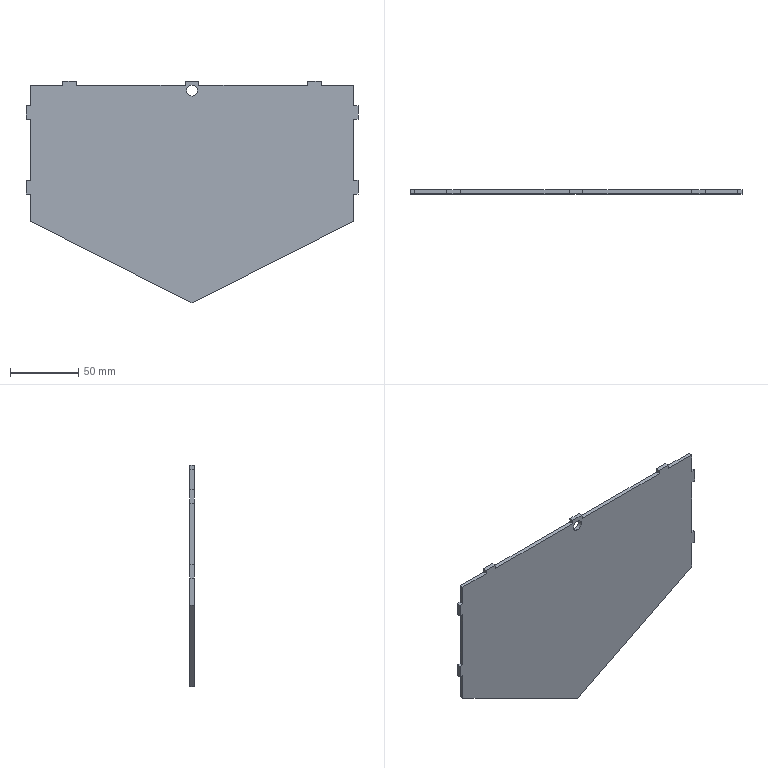Part | SolidWorks | features ICE 2, Extrusion 1 | 1 solid | 37 faces | box 244 x 3 x 163 mm | volume 93299 mm3 | plane 35 | cylinder 2 | commonest cylinder face diameters 8 x2
STEP:
#1=CARTESIAN_POINT('',(0.,0.,42.));
#2=VERTEX_POINT('',#1);
#3=CARTESIAN_POINT('',(0.,0.,50.));
#4=VERTEX_POINT('',#3);
#5=CARTESIAN_POINT('',(0.,0.,46.));
#6=DIRECTION('',(0.,1.,0.));
#7=DIRECTION('',(0.,0.,1.));
#8=AXIS2_PLACEMENT_3D('',#5,#6,#7);
#9=CIRCLE('',#8,4.);
#10=EDGE_CURVE('',#2,#4,#9,.T.);
#11=ORIENTED_EDGE('',*,*,#10,.F.);
#12=CARTESIAN_POINT('',(0.,3.,42.));
#13=VERTEX_POINT('',#12);
#14=CARTESIAN_POINT('',(0.,0.,42.));
#15=DIRECTION('',(0.,1.,0.));
#16=VECTOR('',#15,1000.);
#17=LINE('',#14,#16);
#18=EDGE_CURVE('',#2,#13,#17,.T.);
#19=ORIENTED_EDGE('',*,*,#18,.T.);
#20=CARTESIAN_POINT('',(0.,3.,50.));
#21=VERTEX_POINT('',#20);
#22=CARTESIAN_POINT('',(0.,3.,46.));
#23=DIRECTION('',(0.,1.,0.));
#24=DIRECTION('',(0.,0.,1.));
#25=AXIS2_PLACEMENT_3D('',#22,#23,#24);
#26=CIRCLE('',#25,4.);
#27=EDGE_CURVE('',#13,#21,#26,.T.);
#28=ORIENTED_EDGE('',*,*,#27,.T.);
#29=CARTESIAN_POINT('',(0.,0.,50.));
#30=DIRECTION('',(0.,1.,0.));
#31=VECTOR('',#30,1000.);
#32=LINE('',#29,#31);
#33=EDGE_CURVE('',#4,#21,#32,.T.);
#34=ORIENTED_EDGE('',*,*,#33,.F.);
#35=EDGE_LOOP('',(#11,#19,#28,#34));
#36=FACE_OUTER_BOUND('',#35,.T.);
#37=CARTESIAN_POINT('',(0.,0.,46.));
#38=DIRECTION('',(0.,1.,0.));
#39=DIRECTION('',(0.,0.,1.));
#40=AXIS2_PLACEMENT_3D('',#37,#38,#39);
#41=CYLINDRICAL_SURFACE('',#40,4.);
#42=ADVANCED_FACE('',(#36),#41,.F.);
#43=CARTESIAN_POINT('',(5.,3.,50.));
#44=VERTEX_POINT('',#43);
#45=CARTESIAN_POINT('',(85.,3.,50.));
#46=VERTEX_POINT('',#45);
#47=CARTESIAN_POINT('',(-119.,3.,50.));
#48=DIRECTION('',(1.,0.,0.));
#49=VECTOR('',#48,1000.);
#50=LINE('',#47,#49);
#51=EDGE_CURVE('',#44,#46,#50,.T.);
#52=ORIENTED_EDGE('',*,*,#51,.F.);
#53=CARTESIAN_POINT('',(5.,0.,50.));
#54=VERTEX_POINT('',#53);
#55=CARTESIAN_POINT('',(5.,-10.44,50.));
#56=DIRECTION('',(0.,1.,0.));
#57=VECTOR('',#56,1000.);
#58=LINE('',#55,#57);
#59=EDGE_CURVE('',#54,#44,#58,.T.);
#60=ORIENTED_EDGE('',*,*,#59,.F.);
#61=CARTESIAN_POINT('',(85.,0.,50.));
#62=VERTEX_POINT('',#61);
#63=CARTESIAN_POINT('',(-119.,0.,50.));
#64=DIRECTION('',(1.,0.,0.));
#65=VECTOR('',#64,1000.);
#66=LINE('',#63,#65);
#67=EDGE_CURVE('',#54,#62,#66,.T.);
#68=ORIENTED_EDGE('',*,*,#67,.T.);
#69=CARTESIAN_POINT('',(85.,-10.44,50.));
#70=DIRECTION('',(0.,1.,0.));
#71=VECTOR('',#70,1000.);
#72=LINE('',#69,#71);
#73=EDGE_CURVE('',#62,#46,#72,.T.);
#74=ORIENTED_EDGE('',*,*,#73,.T.);
#75=EDGE_LOOP('',(#52,#60,#68,#74));
#76=FACE_OUTER_BOUND('',#75,.T.);
#77=CARTESIAN_POINT('',(-119.,3.,50.));
#78=DIRECTION('',(0.,0.,-1.));
#79=DIRECTION('',(-1.,0.,0.));
#80=AXIS2_PLACEMENT_3D('',#77,#78,#79);
#81=PLANE('',#80);
#82=ADVANCED_FACE('',(#76),#81,.F.);
#83=CARTESIAN_POINT('',(-85.,0.,50.));
#84=VERTEX_POINT('',#83);
#85=CARTESIAN_POINT('',(-5.,0.,50.));
#86=VERTEX_POINT('',#85);
#87=CARTESIAN_POINT('',(-119.,0.,50.));
#88=DIRECTION('',(1.,0.,0.));
#89=VECTOR('',#88,1000.);
#90=LINE('',#87,#89);
#91=EDGE_CURVE('',#84,#86,#90,.T.);
#92=ORIENTED_EDGE('',*,*,#91,.T.);
#93=CARTESIAN_POINT('',(-5.,3.,50.));
#94=VERTEX_POINT('',#93);
#95=CARTESIAN_POINT('',(-5.,-10.44,50.));
#96=DIRECTION('',(0.,1.,0.));
#97=VECTOR('',#96,1000.);
#98=LINE('',#95,#97);
#99=EDGE_CURVE('',#86,#94,#98,.T.);
#100=ORIENTED_EDGE('',*,*,#99,.T.);
#101=CARTESIAN_POINT('',(-85.,3.,50.));
#102=VERTEX_POINT('',#101);
#103=CARTESIAN_POINT('',(-119.,3.,50.));
#104=DIRECTION('',(1.,0.,0.));
#105=VECTOR('',#104,1000.);
#106=LINE('',#103,#105);
#107=EDGE_CURVE('',#102,#94,#106,.T.);
#108=ORIENTED_EDGE('',*,*,#107,.F.);
#109=CARTESIAN_POINT('',(-85.,-10.44,50.));
#110=DIRECTION('',(0.,1.,0.));
#111=VECTOR('',#110,1000.);
#112=LINE('',#109,#111);
#113=EDGE_CURVE('',#84,#102,#112,.T.);
#114=ORIENTED_EDGE('',*,*,#113,.F.);
#115=EDGE_LOOP('',(#92,#100,#108,#114));
#116=FACE_OUTER_BOUND('',#115,.T.);
#117=CARTESIAN_POINT('',(-119.,3.,50.));
#118=DIRECTION('',(0.,0.,-1.));
#119=DIRECTION('',(-1.,0.,0.));
#120=AXIS2_PLACEMENT_3D('',#117,#118,#119);
#121=PLANE('',#120);
#122=ADVANCED_FACE('',(#116),#121,.F.);
#123=CARTESIAN_POINT('',(95.,0.,50.));
#124=VERTEX_POINT('',#123);
#125=CARTESIAN_POINT('',(95.,3.,50.));
#126=VERTEX_POINT('',#125);
#127=CARTESIAN_POINT('',(95.,-10.44,50.));
#128=DIRECTION('',(0.,1.,0.));
#129=VECTOR('',#128,1000.);
#130=LINE('',#127,#129);
#131=EDGE_CURVE('',#124,#126,#130,.T.);
#132=ORIENTED_EDGE('',*,*,#131,.F.);
#133=CARTESIAN_POINT('',(119.,0.,50.));
#134=VERTEX_POINT('',#133);
#135=CARTESIAN_POINT('',(-119.,0.,50.));
#136=DIRECTION('',(1.,0.,0.));
#137=VECTOR('',#136,1000.);
#138=LINE('',#135,#137);
#139=EDGE_CURVE('',#124,#134,#138,.T.);
#140=ORIENTED_EDGE('',*,*,#139,.T.);
#141=CARTESIAN_POINT('',(119.,3.,50.));
#142=VERTEX_POINT('',#141);
#143=CARTESIAN_POINT('',(119.,3.,50.));
#144=DIRECTION('',(0.,-1.,0.));
#145=VECTOR('',#144,1000.);
#146=LINE('',#143,#145);
#147=EDGE_CURVE('',#142,#134,#146,.T.);
#148=ORIENTED_EDGE('',*,*,#147,.F.);
#149=CARTESIAN_POINT('',(-119.,3.,50.));
#150=DIRECTION('',(1.,0.,0.));
#151=VECTOR('',#150,1000.);
#152=LINE('',#149,#151);
#153=EDGE_CURVE('',#126,#142,#152,.T.);
#154=ORIENTED_EDGE('',*,*,#153,.F.);
#155=EDGE_LOOP('',(#132,#140,#148,#154));
#156=FACE_OUTER_BOUND('',#155,.T.);
#157=CARTESIAN_POINT('',(-119.,3.,50.));
#158=DIRECTION('',(0.,0.,-1.));
#159=DIRECTION('',(-1.,0.,0.));
#160=AXIS2_PLACEMENT_3D('',#157,#158,#159);
#161=PLANE('',#160);
#162=ADVANCED_FACE('',(#156),#161,.F.);
#163=CARTESIAN_POINT('',(-119.,0.,-50.));
#164=VERTEX_POINT('',#163);
#165=CARTESIAN_POINT('',(-119.,0.,-30.));
#166=VERTEX_POINT('',#165);
#167=CARTESIAN_POINT('',(-119.,0.,50.));
#168=DIRECTION('',(0.,0.,1.));
#169=VECTOR('',#168,1000.);
#170=LINE('',#167,#169);
#171=EDGE_CURVE('',#164,#166,#170,.T.);
#172=ORIENTED_EDGE('',*,*,#171,.T.);
#173=CARTESIAN_POINT('',(-119.,3.,-30.));
#174=VERTEX_POINT('',#173);
#175=CARTESIAN_POINT('',(-119.,-10.44,-30.));
#176=DIRECTION('',(0.,1.,0.));
#177=VECTOR('',#176,1000.);
#178=LINE('',#175,#177);
#179=EDGE_CURVE('',#166,#174,#178,.T.);
#180=ORIENTED_EDGE('',*,*,#179,.T.);
#181=CARTESIAN_POINT('',(-119.,3.,-50.));
#182=VERTEX_POINT('',#181);
#183=CARTESIAN_POINT('',(-119.,3.,50.));
#184=DIRECTION('',(0.,0.,1.));
#185=VECTOR('',#184,1000.);
#186=LINE('',#183,#185);
#187=EDGE_CURVE('',#182,#174,#186,.T.);
#188=ORIENTED_EDGE('',*,*,#187,.F.);
#189=CARTESIAN_POINT('',(-119.,3.,-50.));
#190=DIRECTION('',(0.,-1.,0.));
#191=VECTOR('',#190,1000.);
#192=LINE('',#189,#191);
#193=EDGE_CURVE('',#182,#164,#192,.T.);
#194=ORIENTED_EDGE('',*,*,#193,.T.);
#195=EDGE_LOOP('',(#172,#180,#188,#194));
#196=FACE_OUTER_BOUND('',#195,.T.);
#197=CARTESIAN_POINT('',(-119.,3.,50.));
#198=DIRECTION('',(1.,0.,0.));
#199=DIRECTION('',(0.,0.,-1.));
#200=AXIS2_PLACEMENT_3D('',#197,#198,#199);
#201=PLANE('',#200);
#202=ADVANCED_FACE('',(#196),#201,.F.);
#203=CARTESIAN_POINT('',(-119.,0.,35.));
#204=VERTEX_POINT('',#203);
#205=CARTESIAN_POINT('',(-119.,3.,35.));
#206=VERTEX_POINT('',#205);
#207=CARTESIAN_POINT('',(-119.,-10.44,35.));
#208=DIRECTION('',(0.,1.,0.));
#209=VECTOR('',#208,1000.);
#210=LINE('',#207,#209);
#211=EDGE_CURVE('',#204,#206,#210,.T.);
#212=ORIENTED_EDGE('',*,*,#211,.F.);
#213=CARTESIAN_POINT('',(-119.,0.,50.));
#214=VERTEX_POINT('',#213);
#215=CARTESIAN_POINT('',(-119.,0.,50.));
#216=DIRECTION('',(0.,0.,1.));
#217=VECTOR('',#216,1000.);
#218=LINE('',#215,#217);
#219=EDGE_CURVE('',#204,#214,#218,.T.);
#220=ORIENTED_EDGE('',*,*,#219,.T.);
#221=CARTESIAN_POINT('',(-119.,3.,50.));
#222=VERTEX_POINT('',#221);
#223=CARTESIAN_POINT('',(-119.,3.,50.));
#224=DIRECTION('',(0.,-1.,0.));
#225=VECTOR('',#224,1000.);
#226=LINE('',#223,#225);
#227=EDGE_CURVE('',#222,#214,#226,.T.);
#228=ORIENTED_EDGE('',*,*,#227,.F.);
#229=CARTESIAN_POINT('',(-119.,3.,50.));
#230=DIRECTION('',(0.,0.,1.));
#231=VECTOR('',#230,1000.);
#232=LINE('',#229,#231);
#233=EDGE_CURVE('',#206,#222,#232,.T.);
#234=ORIENTED_EDGE('',*,*,#233,.F.);
#235=EDGE_LOOP('',(#212,#220,#228,#234));
#236=FACE_OUTER_BOUND('',#235,.T.);
#237=CARTESIAN_POINT('',(-119.,3.,50.));
#238=DIRECTION('',(1.,0.,0.));
#239=DIRECTION('',(0.,0.,-1.));
#240=AXIS2_PLACEMENT_3D('',#237,#238,#239);
#241=PLANE('',#240);
#242=ADVANCED_FACE('',(#236),#241,.F.);
#243=CARTESIAN_POINT('',(119.,3.,25.));
#244=VERTEX_POINT('',#243);
#245=CARTESIAN_POINT('',(119.,3.,-20.));
#246=VERTEX_POINT('',#245);
#247=CARTESIAN_POINT('',(119.,3.,50.));
#248=DIRECTION('',(0.,0.,-1.));
#249=VECTOR('',#248,1000.);
#250=LINE('',#247,#249);
#251=EDGE_CURVE('',#244,#246,#250,.T.);
#252=ORIENTED_EDGE('',*,*,#251,.F.);
#253=CARTESIAN_POINT('',(119.,0.,25.));
#254=VERTEX_POINT('',#253);
#255=CARTESIAN_POINT('',(119.,-10.44,25.));
#256=DIRECTION('',(0.,1.,0.));
#257=VECTOR('',#256,1000.);
#258=LINE('',#255,#257);
#259=EDGE_CURVE('',#254,#244,#258,.T.);
#260=ORIENTED_EDGE('',*,*,#259,.F.);
#261=CARTESIAN_POINT('',(119.,0.,-20.));
#262=VERTEX_POINT('',#261);
#263=CARTESIAN_POINT('',(119.,0.,50.));
#264=DIRECTION('',(0.,0.,-1.));
#265=VECTOR('',#264,1000.);
#266=LINE('',#263,#265);
#267=EDGE_CURVE('',#254,#262,#266,.T.);
#268=ORIENTED_EDGE('',*,*,#267,.T.);
#269=CARTESIAN_POINT('',(119.,-10.44,-20.));
#270=DIRECTION('',(0.,1.,0.));
#271=VECTOR('',#270,1000.);
#272=LINE('',#269,#271);
#273=EDGE_CURVE('',#262,#246,#272,.T.);
#274=ORIENTED_EDGE('',*,*,#273,.T.);
#275=EDGE_LOOP('',(#252,#260,#268,#274));
#276=FACE_OUTER_BOUND('',#275,.T.);
#277=CARTESIAN_POINT('',(119.,3.,50.));
#278=DIRECTION('',(-1.,0.,0.));
#279=DIRECTION('',(0.,0.,1.));
#280=AXIS2_PLACEMENT_3D('',#277,#278,#279);
#281=PLANE('',#280);
#282=ADVANCED_FACE('',(#276),#281,.F.);
#283=CARTESIAN_POINT('',(119.,0.,-30.));
#284=VERTEX_POINT('',#283);
#285=CARTESIAN_POINT('',(119.,3.,-30.));
#286=VERTEX_POINT('',#285);
#287=CARTESIAN_POINT('',(119.,-10.44,-30.));
#288=DIRECTION('',(0.,1.,0.));
#289=VECTOR('',#288,1000.);
#290=LINE('',#287,#289);
#291=EDGE_CURVE('',#284,#286,#290,.T.);
#292=ORIENTED_EDGE('',*,*,#291,.F.);
#293=CARTESIAN_POINT('',(119.,0.,-50.));
#294=VERTEX_POINT('',#293);
#295=CARTESIAN_POINT('',(119.,0.,50.));
#296=DIRECTION('',(0.,0.,-1.));
#297=VECTOR('',#296,1000.);
#298=LINE('',#295,#297);
#299=EDGE_CURVE('',#284,#294,#298,.T.);
#300=ORIENTED_EDGE('',*,*,#299,.T.);
#301=CARTESIAN_POINT('',(119.,3.,-50.));
#302=VERTEX_POINT('',#301);
#303=CARTESIAN_POINT('',(119.,3.,-50.));
#304=DIRECTION('',(0.,-1.,0.));
#305=VECTOR('',#304,1000.);
#306=LINE('',#303,#305);
#307=EDGE_CURVE('',#302,#294,#306,.T.);
#308=ORIENTED_EDGE('',*,*,#307,.F.);
#309=CARTESIAN_POINT('',(119.,3.,50.));
#310=DIRECTION('',(0.,0.,-1.));
#311=VECTOR('',#310,1000.);
#312=LINE('',#309,#311);
#313=EDGE_CURVE('',#286,#302,#312,.T.);
#314=ORIENTED_EDGE('',*,*,#313,.F.);
#315=EDGE_LOOP('',(#292,#300,#308,#314));
#316=FACE_OUTER_BOUND('',#315,.T.);
#317=CARTESIAN_POINT('',(119.,3.,50.));
#318=DIRECTION('',(-1.,0.,0.));
#319=DIRECTION('',(0.,0.,1.));
#320=AXIS2_PLACEMENT_3D('',#317,#318,#319);
#321=PLANE('',#320);
#322=ADVANCED_FACE('',(#316),#321,.F.);
#323=CARTESIAN_POINT('',(0.,0.,-110.));
#324=VERTEX_POINT('',#323);
#325=CARTESIAN_POINT('',(0.,0.,-110.));
#326=DIRECTION('',(-0.8929,0.,-0.4502));
#327=VECTOR('',#326,1000.);
#328=LINE('',#325,#327);
#329=EDGE_CURVE('',#294,#324,#328,.T.);
#330=ORIENTED_EDGE('',*,*,#329,.T.);
#331=CARTESIAN_POINT('',(0.,3.,-110.));
#332=VERTEX_POINT('',#331);
#333=CARTESIAN_POINT('',(0.,3.,-110.));
#334=DIRECTION('',(0.,-1.,0.));
#335=VECTOR('',#334,1000.);
#336=LINE('',#333,#335);
#337=EDGE_CURVE('',#332,#324,#336,.T.);
#338=ORIENTED_EDGE('',*,*,#337,.F.);
#339=CARTESIAN_POINT('',(0.,3.,-110.));
#340=DIRECTION('',(-0.8929,0.,-0.4502));
#341=VECTOR('',#340,1000.);
#342=LINE('',#339,#341);
#343=EDGE_CURVE('',#302,#332,#342,.T.);
#344=ORIENTED_EDGE('',*,*,#343,.F.);
#345=ORIENTED_EDGE('',*,*,#307,.T.);
#346=EDGE_LOOP('',(#330,#338,#344,#345));
#347=FACE_OUTER_BOUND('',#346,.T.);
#348=CARTESIAN_POINT('',(0.,3.,-110.));
#349=DIRECTION('',(-0.4502,0.,0.8929));
#350=DIRECTION('',(0.8929,0.,0.4502));
#351=AXIS2_PLACEMENT_3D('',#348,#349,#350);
#352=PLANE('',#351);
#353=ADVANCED_FACE('',(#347),#352,.F.);
#354=CARTESIAN_POINT('',(-119.,0.,-50.));
#355=DIRECTION('',(-0.8929,0.,0.4502));
#356=VECTOR('',#355,1000.);
#357=LINE('',#354,#356);
#358=EDGE_CURVE('',#324,#164,#357,.T.);
#359=ORIENTED_EDGE('',*,*,#358,.T.);
#360=ORIENTED_EDGE('',*,*,#193,.F.);
#361=CARTESIAN_POINT('',(-119.,3.,-50.));
#362=DIRECTION('',(-0.8929,0.,0.4502));
#363=VECTOR('',#362,1000.);
#364=LINE('',#361,#363);
#365=EDGE_CURVE('',#332,#182,#364,.T.);
#366=ORIENTED_EDGE('',*,*,#365,.F.);
#367=ORIENTED_EDGE('',*,*,#337,.T.);
#368=EDGE_LOOP('',(#359,#360,#366,#367));
#369=FACE_OUTER_BOUND('',#368,.T.);
#370=CARTESIAN_POINT('',(-119.,3.,-50.));
#371=DIRECTION('',(0.4502,0.,0.8929));
#372=DIRECTION('',(0.8929,0.,-0.4502));
#373=AXIS2_PLACEMENT_3D('',#370,#371,#372);
#374=PLANE('',#373);
#375=ADVANCED_FACE('',(#369),#374,.F.);
#376=CARTESIAN_POINT('',(-119.,3.,-20.));
#377=VERTEX_POINT('',#376);
#378=CARTESIAN_POINT('',(-119.,3.,25.));
#379=VERTEX_POINT('',#378);
#380=CARTESIAN_POINT('',(-119.,3.,50.));
#381=DIRECTION('',(0.,0.,1.));
#382=VECTOR('',#381,1000.);
#383=LINE('',#380,#382);
#384=EDGE_CURVE('',#377,#379,#383,.T.);
#385=ORIENTED_EDGE('',*,*,#384,.F.);
#386=CARTESIAN_POINT('',(-119.,0.,-20.));
#387=VERTEX_POINT('',#386);
#388=CARTESIAN_POINT('',(-119.,-10.44,-20.));
#389=DIRECTION('',(0.,1.,0.));
#390=VECTOR('',#389,1000.);
#391=LINE('',#388,#390);
#392=EDGE_CURVE('',#387,#377,#391,.T.);
#393=ORIENTED_EDGE('',*,*,#392,.F.);
#394=CARTESIAN_POINT('',(-119.,0.,25.));
#395=VERTEX_POINT('',#394);
#396=CARTESIAN_POINT('',(-119.,0.,50.));
#397=DIRECTION('',(0.,0.,1.));
#398=VECTOR('',#397,1000.);
#399=LINE('',#396,#398);
#400=EDGE_CURVE('',#387,#395,#399,.T.);
#401=ORIENTED_EDGE('',*,*,#400,.T.);
#402=CARTESIAN_POINT('',(-119.,-10.44,25.));
#403=DIRECTION('',(0.,1.,0.));
#404=VECTOR('',#403,1000.);
#405=LINE('',#402,#404);
#406=EDGE_CURVE('',#395,#379,#405,.T.);
#407=ORIENTED_EDGE('',*,*,#406,.T.);
#408=EDGE_LOOP('',(#385,#393,#401,#407));
#409=FACE_OUTER_BOUND('',#408,.T.);
#410=CARTESIAN_POINT('',(-119.,3.,50.));
#411=DIRECTION('',(1.,0.,0.));
#412=DIRECTION('',(0.,0.,-1.));
#413=AXIS2_PLACEMENT_3D('',#410,#411,#412);
#414=PLANE('',#413);
#415=ADVANCED_FACE('',(#409),#414,.F.);
#416=CARTESIAN_POINT('',(-95.,0.,50.));
#417=VERTEX_POINT('',#416);
#418=CARTESIAN_POINT('',(-119.,0.,50.));
#419=DIRECTION('',(1.,0.,0.));
#420=VECTOR('',#419,1000.);
#421=LINE('',#418,#420);
#422=EDGE_CURVE('',#214,#417,#421,.T.);
#423=ORIENTED_EDGE('',*,*,#422,.T.);
#424=CARTESIAN_POINT('',(-95.,3.,50.));
#425=VERTEX_POINT('',#424);
#426=CARTESIAN_POINT('',(-95.,-10.44,50.));
#427=DIRECTION('',(0.,1.,0.));
#428=VECTOR('',#427,1000.);
#429=LINE('',#426,#428);
#430=EDGE_CURVE('',#417,#425,#429,.T.);
#431=ORIENTED_EDGE('',*,*,#430,.T.);
#432=CARTESIAN_POINT('',(-119.,3.,50.));
#433=DIRECTION('',(1.,0.,0.));
#434=VECTOR('',#433,1000.);
#435=LINE('',#432,#434);
#436=EDGE_CURVE('',#222,#425,#435,.T.);
#437=ORIENTED_EDGE('',*,*,#436,.F.);
#438=ORIENTED_EDGE('',*,*,#227,.T.);
#439=EDGE_LOOP('',(#423,#431,#437,#438));
#440=FACE_OUTER_BOUND('',#439,.T.);
#441=CARTESIAN_POINT('',(-119.,3.,50.));
#442=DIRECTION('',(0.,0.,-1.));
#443=DIRECTION('',(-1.,0.,0.));
#444=AXIS2_PLACEMENT_3D('',#441,#442,#443);
#445=PLANE('',#444);
#446=ADVANCED_FACE('',(#440),#445,.F.);
#447=CARTESIAN_POINT('',(119.,0.,35.));
#448=VERTEX_POINT('',#447);
#449=CARTESIAN_POINT('',(119.,0.,50.));
#450=DIRECTION('',(0.,0.,-1.));
#451=VECTOR('',#450,1000.);
#452=LINE('',#449,#451);
#453=EDGE_CURVE('',#134,#448,#452,.T.);
#454=ORIENTED_EDGE('',*,*,#453,.T.);
#455=CARTESIAN_POINT('',(119.,3.,35.));
#456=VERTEX_POINT('',#455);
#457=CARTESIAN_POINT('',(119.,-10.44,35.));
#458=DIRECTION('',(0.,1.,0.));
#459=VECTOR('',#458,1000.);
#460=LINE('',#457,#459);
#461=EDGE_CURVE('',#448,#456,#460,.T.);
#462=ORIENTED_EDGE('',*,*,#461,.T.);
#463=CARTESIAN_POINT('',(119.,3.,50.));
#464=DIRECTION('',(0.,0.,-1.));
#465=VECTOR('',#464,1000.);
#466=LINE('',#463,#465);
#467=EDGE_CURVE('',#142,#456,#466,.T.);
#468=ORIENTED_EDGE('',*,*,#467,.F.);
#469=ORIENTED_EDGE('',*,*,#147,.T.);
#470=EDGE_LOOP('',(#454,#462,#468,#469));
#471=FACE_OUTER_BOUND('',#470,.T.);
#472=CARTESIAN_POINT('',(119.,3.,50.));
#473=DIRECTION('',(-1.,0.,0.));
#474=DIRECTION('',(0.,0.,1.));
#475=AXIS2_PLACEMENT_3D('',#472,#473,#474);
#476=PLANE('',#475);
#477=ADVANCED_FACE('',(#471),#476,.F.);
#478=CARTESIAN_POINT('',(0.,3.,46.));
#479=DIRECTION('',(0.,1.,0.));
#480=DIRECTION('',(0.,0.,1.));
#481=AXIS2_PLACEMENT_3D('',#478,#479,#480);
#482=CIRCLE('',#481,4.);
#483=EDGE_CURVE('',#21,#13,#482,.T.);
#484=ORIENTED_EDGE('',*,*,#483,.F.);
#485=ORIENTED_EDGE('',*,*,#27,.F.);
#486=EDGE_LOOP('',(#484,#485));
#487=FACE_BOUND('',#486,.T.);
#488=ORIENTED_EDGE('',*,*,#343,.T.);
#489=ORIENTED_EDGE('',*,*,#365,.T.);
#490=ORIENTED_EDGE('',*,*,#187,.T.);
#491=CARTESIAN_POINT('',(-122.,3.,-30.));
#492=VERTEX_POINT('',#491);
#493=CARTESIAN_POINT('',(-119.,3.,-30.));
#494=DIRECTION('',(-1.,0.,0.));
#495=VECTOR('',#494,1000.);
#496=LINE('',#493,#495);
#497=EDGE_CURVE('',#174,#492,#496,.T.);
#498=ORIENTED_EDGE('',*,*,#497,.T.);
#499=CARTESIAN_POINT('',(-122.,3.,-20.));
#500=VERTEX_POINT('',#499);
#501=CARTESIAN_POINT('',(-122.,3.,-30.));
#502=DIRECTION('',(0.,0.,1.));
#503=VECTOR('',#502,1000.);
#504=LINE('',#501,#503);
#505=EDGE_CURVE('',#492,#500,#504,.T.);
#506=ORIENTED_EDGE('',*,*,#505,.T.);
#507=CARTESIAN_POINT('',(-119.,3.,-20.));
#508=DIRECTION('',(1.,0.,0.));
#509=VECTOR('',#508,1000.);
#510=LINE('',#507,#509);
#511=EDGE_CURVE('',#500,#377,#510,.T.);
#512=ORIENTED_EDGE('',*,*,#511,.T.);
#513=ORIENTED_EDGE('',*,*,#384,.T.);
#514=CARTESIAN_POINT('',(-122.,3.,25.));
#515=VERTEX_POINT('',#514);
#516=CARTESIAN_POINT('',(-119.,3.,25.));
#517=DIRECTION('',(-1.,0.,0.));
#518=VECTOR('',#517,1000.);
#519=LINE('',#516,#518);
#520=EDGE_CURVE('',#379,#515,#519,.T.);
#521=ORIENTED_EDGE('',*,*,#520,.T.);
#522=CARTESIAN_POINT('',(-122.,3.,35.));
#523=VERTEX_POINT('',#522);
#524=CARTESIAN_POINT('',(-122.,3.,35.));
#525=DIRECTION('',(0.,0.,1.));
#526=VECTOR('',#525,1000.);
#527=LINE('',#524,#526);
#528=EDGE_CURVE('',#515,#523,#527,.T.);
#529=ORIENTED_EDGE('',*,*,#528,.T.);
#530=CARTESIAN_POINT('',(-119.,3.,35.));
#531=DIRECTION('',(1.,0.,0.));
#532=VECTOR('',#531,1000.);
#533=LINE('',#530,#532);
#534=EDGE_CURVE('',#523,#206,#533,.T.);
#535=ORIENTED_EDGE('',*,*,#534,.T.);
#536=ORIENTED_EDGE('',*,*,#233,.T.);
#537=ORIENTED_EDGE('',*,*,#436,.T.);
#538=CARTESIAN_POINT('',(-95.,3.,53.));
#539=VERTEX_POINT('',#538);
#540=CARTESIAN_POINT('',(-95.,3.,50.));
#541=DIRECTION('',(0.,0.,1.));
#542=VECTOR('',#541,1000.);
#543=LINE('',#540,#542);
#544=EDGE_CURVE('',#425,#539,#543,.T.);
#545=ORIENTED_EDGE('',*,*,#544,.T.);
#546=CARTESIAN_POINT('',(-85.,3.,53.));
#547=VERTEX_POINT('',#546);
#548=CARTESIAN_POINT('',(-85.,3.,53.));
#549=DIRECTION('',(1.,0.,0.));
#550=VECTOR('',#549,1000.);
#551=LINE('',#548,#550);
#552=EDGE_CURVE('',#539,#547,#551,.T.);
#553=ORIENTED_EDGE('',*,*,#552,.T.);
#554=CARTESIAN_POINT('',(-85.,3.,50.));
#555=DIRECTION('',(0.,0.,-1.));
#556=VECTOR('',#555,1000.);
#557=LINE('',#554,#556);
#558=EDGE_CURVE('',#547,#102,#557,.T.);
#559=ORIENTED_EDGE('',*,*,#558,.T.);
#560=ORIENTED_EDGE('',*,*,#107,.T.);
#561=CARTESIAN_POINT('',(-5.,3.,53.));
#562=VERTEX_POINT('',#561);
#563=CARTESIAN_POINT('',(-5.,3.,53.));
#564=DIRECTION('',(0.,0.,1.));
#565=VECTOR('',#564,1000.);
#566=LINE('',#563,#565);
#567=EDGE_CURVE('',#94,#562,#566,.T.);
#568=ORIENTED_EDGE('',*,*,#567,.T.);
#569=CARTESIAN_POINT('',(5.,3.,53.));
#570=VERTEX_POINT('',#569);
#571=CARTESIAN_POINT('',(-5.,3.,53.));
#572=DIRECTION('',(1.,0.,0.));
#573=VECTOR('',#572,1000.);
#574=LINE('',#571,#573);
#575=EDGE_CURVE('',#562,#570,#574,.T.);
#576=ORIENTED_EDGE('',*,*,#575,.T.);
#577=CARTESIAN_POINT('',(5.,3.,53.));
#578=DIRECTION('',(0.,0.,-1.));
#579=VECTOR('',#578,1000.);
#580=LINE('',#577,#579);
#581=EDGE_CURVE('',#570,#44,#580,.T.);
#582=ORIENTED_EDGE('',*,*,#581,.T.);
#583=ORIENTED_EDGE('',*,*,#51,.T.);
#584=CARTESIAN_POINT('',(85.,3.,53.));
#585=VERTEX_POINT('',#584);
#586=CARTESIAN_POINT('',(85.,3.,50.));
#587=DIRECTION('',(0.,0.,1.));
#588=VECTOR('',#587,1000.);
#589=LINE('',#586,#588);
#590=EDGE_CURVE('',#46,#585,#589,.T.);
#591=ORIENTED_EDGE('',*,*,#590,.T.);
#592=CARTESIAN_POINT('',(95.,3.,53.));
#593=VERTEX_POINT('',#592);
#594=CARTESIAN_POINT('',(85.,3.,53.));
#595=DIRECTION('',(1.,0.,0.));
#596=VECTOR('',#595,1000.);
#597=LINE('',#594,#596);
#598=EDGE_CURVE('',#585,#593,#597,.T.);
#599=ORIENTED_EDGE('',*,*,#598,.T.);
#600=CARTESIAN_POINT('',(95.,3.,50.));
#601=DIRECTION('',(0.,0.,-1.));
#602=VECTOR('',#601,1000.);
#603=LINE('',#600,#602);
#604=EDGE_CURVE('',#593,#126,#603,.T.);
#605=ORIENTED_EDGE('',*,*,#604,.T.);
#606=ORIENTED_EDGE('',*,*,#153,.T.);
#607=ORIENTED_EDGE('',*,*,#467,.T.);
#608=CARTESIAN_POINT('',(122.,3.,35.));
#609=VERTEX_POINT('',#608);
#610=CARTESIAN_POINT('',(119.,3.,35.));
#611=DIRECTION('',(1.,0.,0.));
#612=VECTOR('',#611,1000.);
#613=LINE('',#610,#612);
#614=EDGE_CURVE('',#456,#609,#613,.T.);
#615=ORIENTED_EDGE('',*,*,#614,.T.);
#616=CARTESIAN_POINT('',(122.,3.,25.));
#617=VERTEX_POINT('',#616);
#618=CARTESIAN_POINT('',(122.,3.,35.));
#619=DIRECTION('',(0.,0.,-1.));
#620=VECTOR('',#619,1000.);
#621=LINE('',#618,#620);
#622=EDGE_CURVE('',#609,#617,#621,.T.);
#623=ORIENTED_EDGE('',*,*,#622,.T.);
#624=CARTESIAN_POINT('',(119.,3.,25.));
#625=DIRECTION('',(-1.,0.,0.));
#626=VECTOR('',#625,1000.);
#627=LINE('',#624,#626);
#628=EDGE_CURVE('',#617,#244,#627,.T.);
#629=ORIENTED_EDGE('',*,*,#628,.T.);
#630=ORIENTED_EDGE('',*,*,#251,.T.);
#631=CARTESIAN_POINT('',(122.,3.,-20.));
#632=VERTEX_POINT('',#631);
#633=CARTESIAN_POINT('',(119.,3.,-20.));
#634=DIRECTION('',(1.,0.,0.));
#635=VECTOR('',#634,1000.);
#636=LINE('',#633,#635);
#637=EDGE_CURVE('',#246,#632,#636,.T.);
#638=ORIENTED_EDGE('',*,*,#637,.T.);
#639=CARTESIAN_POINT('',(122.,3.,-30.));
#640=VERTEX_POINT('',#639);
#641=CARTESIAN_POINT('',(122.,3.,-30.));
#642=DIRECTION('',(0.,0.,-1.));
#643=VECTOR('',#642,1000.);
#644=LINE('',#641,#643);
#645=EDGE_CURVE('',#632,#640,#644,.T.);
#646=ORIENTED_EDGE('',*,*,#645,.T.);
#647=CARTESIAN_POINT('',(119.,3.,-30.));
#648=DIRECTION('',(-1.,0.,0.));
#649=VECTOR('',#648,1000.);
#650=LINE('',#647,#649);
#651=EDGE_CURVE('',#640,#286,#650,.T.);
#652=ORIENTED_EDGE('',*,*,#651,.T.);
#653=ORIENTED_EDGE('',*,*,#313,.T.);
#654=EDGE_LOOP('',(#488,#489,#490,#498,#506,#512,#513,#521,#529,#535,#536,#537,#545,#553,#559,#560,#568,#576,#582,#583,#591,#599,#605,#606,#607,#615,#623,#629,#630,#638,#646,#652,#653));
#655=FACE_OUTER_BOUND('',#654,.T.);
#656=CARTESIAN_POINT('',(0.,3.,0.));
#657=DIRECTION('',(0.,1.,0.));
#658=DIRECTION('',(0.,0.,1.));
#659=AXIS2_PLACEMENT_3D('',#656,#657,#658);
#660=PLANE('',#659);
#661=ADVANCED_FACE('',(#487,#655),#660,.T.);
#662=CARTESIAN_POINT('',(0.,0.,46.));
#663=DIRECTION('',(0.,1.,0.));
#664=DIRECTION('',(0.,0.,1.));
#665=AXIS2_PLACEMENT_3D('',#662,#663,#664);
#666=CIRCLE('',#665,4.);
#667=EDGE_CURVE('',#4,#2,#666,.T.);
#668=ORIENTED_EDGE('',*,*,#667,.T.);
#669=ORIENTED_EDGE('',*,*,#10,.T.);
#670=EDGE_LOOP('',(#668,#669));
#671=FACE_BOUND('',#670,.T.);
#672=ORIENTED_EDGE('',*,*,#329,.F.);
#673=ORIENTED_EDGE('',*,*,#299,.F.);
#674=CARTESIAN_POINT('',(122.,0.,-30.));
#675=VERTEX_POINT('',#674);
#676=CARTESIAN_POINT('',(119.,0.,-30.));
#677=DIRECTION('',(1.,0.,0.));
#678=VECTOR('',#677,1000.);
#679=LINE('',#676,#678);
#680=EDGE_CURVE('',#284,#675,#679,.T.);
#681=ORIENTED_EDGE('',*,*,#680,.T.);
#682=CARTESIAN_POINT('',(122.,0.,-20.));
#683=VERTEX_POINT('',#682);
#684=CARTESIAN_POINT('',(122.,0.,-30.));
#685=DIRECTION('',(0.,0.,1.));
#686=VECTOR('',#685,1000.);
#687=LINE('',#684,#686);
#688=EDGE_CURVE('',#675,#683,#687,.T.);
#689=ORIENTED_EDGE('',*,*,#688,.T.);
#690=CARTESIAN_POINT('',(119.,0.,-20.));
#691=DIRECTION('',(-1.,0.,0.));
#692=VECTOR('',#691,1000.);
#693=LINE('',#690,#692);
#694=EDGE_CURVE('',#683,#262,#693,.T.);
#695=ORIENTED_EDGE('',*,*,#694,.T.);
#696=ORIENTED_EDGE('',*,*,#267,.F.);
#697=CARTESIAN_POINT('',(122.,0.,25.));
#698=VERTEX_POINT('',#697);
#699=CARTESIAN_POINT('',(119.,0.,25.));
#700=DIRECTION('',(1.,0.,0.));
#701=VECTOR('',#700,1000.);
#702=LINE('',#699,#701);
#703=EDGE_CURVE('',#254,#698,#702,.T.);
#704=ORIENTED_EDGE('',*,*,#703,.T.);
#705=CARTESIAN_POINT('',(122.,0.,35.));
#706=VERTEX_POINT('',#705);
#707=CARTESIAN_POINT('',(122.,0.,35.));
#708=DIRECTION('',(0.,0.,1.));
#709=VECTOR('',#708,1000.);
#710=LINE('',#707,#709);
#711=EDGE_CURVE('',#698,#706,#710,.T.);
#712=ORIENTED_EDGE('',*,*,#711,.T.);
#713=CARTESIAN_POINT('',(119.,0.,35.));
#714=DIRECTION('',(-1.,0.,0.));
#715=VECTOR('',#714,1000.);
#716=LINE('',#713,#715);
#717=EDGE_CURVE('',#706,#448,#716,.T.);
#718=ORIENTED_EDGE('',*,*,#717,.T.);
#719=ORIENTED_EDGE('',*,*,#453,.F.);
#720=ORIENTED_EDGE('',*,*,#139,.F.);
#721=CARTESIAN_POINT('',(95.,0.,53.));
#722=VERTEX_POINT('',#721);
#723=CARTESIAN_POINT('',(95.,0.,50.));
#724=DIRECTION('',(0.,0.,1.));
#725=VECTOR('',#724,1000.);
#726=LINE('',#723,#725);
#727=EDGE_CURVE('',#124,#722,#726,.T.);
#728=ORIENTED_EDGE('',*,*,#727,.T.);
#729=CARTESIAN_POINT('',(85.,0.,53.));
#730=VERTEX_POINT('',#729);
#731=CARTESIAN_POINT('',(85.,0.,53.));
#732=DIRECTION('',(-1.,0.,0.));
#733=VECTOR('',#732,1000.);
#734=LINE('',#731,#733);
#735=EDGE_CURVE('',#722,#730,#734,.T.);
#736=ORIENTED_EDGE('',*,*,#735,.T.);
#737=CARTESIAN_POINT('',(85.,0.,50.));
#738=DIRECTION('',(0.,0.,-1.));
#739=VECTOR('',#738,1000.);
#740=LINE('',#737,#739);
#741=EDGE_CURVE('',#730,#62,#740,.T.);
#742=ORIENTED_EDGE('',*,*,#741,.T.);
#743=ORIENTED_EDGE('',*,*,#67,.F.);
#744=CARTESIAN_POINT('',(5.,0.,53.));
#745=VERTEX_POINT('',#744);
#746=CARTESIAN_POINT('',(5.,0.,53.));
#747=DIRECTION('',(0.,0.,1.));
#748=VECTOR('',#747,1000.);
#749=LINE('',#746,#748);
#750=EDGE_CURVE('',#54,#745,#749,.T.);
#751=ORIENTED_EDGE('',*,*,#750,.T.);
#752=CARTESIAN_POINT('',(-5.,0.,53.));
#753=VERTEX_POINT('',#752);
#754=CARTESIAN_POINT('',(-5.,0.,53.));
#755=DIRECTION('',(-1.,0.,0.));
#756=VECTOR('',#755,1000.);
#757=LINE('',#754,#756);
#758=EDGE_CURVE('',#745,#753,#757,.T.);
#759=ORIENTED_EDGE('',*,*,#758,.T.);
#760=CARTESIAN_POINT('',(-5.,0.,53.));
#761=DIRECTION('',(0.,0.,-1.));
#762=VECTOR('',#761,1000.);
#763=LINE('',#760,#762);
#764=EDGE_CURVE('',#753,#86,#763,.T.);
#765=ORIENTED_EDGE('',*,*,#764,.T.);
#766=ORIENTED_EDGE('',*,*,#91,.F.);
#767=CARTESIAN_POINT('',(-85.,0.,53.));
#768=VERTEX_POINT('',#767);
#769=CARTESIAN_POINT('',(-85.,0.,50.));
#770=DIRECTION('',(0.,0.,1.));
#771=VECTOR('',#770,1000.);
#772=LINE('',#769,#771);
#773=EDGE_CURVE('',#84,#768,#772,.T.);
#774=ORIENTED_EDGE('',*,*,#773,.T.);
#775=CARTESIAN_POINT('',(-95.,0.,53.));
#776=VERTEX_POINT('',#775);
#777=CARTESIAN_POINT('',(-85.,0.,53.));
#778=DIRECTION('',(-1.,0.,0.));
#779=VECTOR('',#778,1000.);
#780=LINE('',#777,#779);
#781=EDGE_CURVE('',#768,#776,#780,.T.);
#782=ORIENTED_EDGE('',*,*,#781,.T.);
#783=CARTESIAN_POINT('',(-95.,0.,50.));
#784=DIRECTION('',(0.,0.,-1.));
#785=VECTOR('',#784,1000.);
#786=LINE('',#783,#785);
#787=EDGE_CURVE('',#776,#417,#786,.T.);
#788=ORIENTED_EDGE('',*,*,#787,.T.);
#789=ORIENTED_EDGE('',*,*,#422,.F.);
#790=ORIENTED_EDGE('',*,*,#219,.F.);
#791=CARTESIAN_POINT('',(-122.,0.,35.));
#792=VERTEX_POINT('',#791);
#793=CARTESIAN_POINT('',(-119.,0.,35.));
#794=DIRECTION('',(-1.,0.,0.));
#795=VECTOR('',#794,1000.);
#796=LINE('',#793,#795);
#797=EDGE_CURVE('',#204,#792,#796,.T.);
#798=ORIENTED_EDGE('',*,*,#797,.T.);
#799=CARTESIAN_POINT('',(-122.,0.,25.));
#800=VERTEX_POINT('',#799);
#801=CARTESIAN_POINT('',(-122.,0.,35.));
#802=DIRECTION('',(0.,0.,-1.));
#803=VECTOR('',#802,1000.);
#804=LINE('',#801,#803);
#805=EDGE_CURVE('',#792,#800,#804,.T.);
#806=ORIENTED_EDGE('',*,*,#805,.T.);
#807=CARTESIAN_POINT('',(-119.,0.,25.));
#808=DIRECTION('',(1.,0.,0.));
#809=VECTOR('',#808,1000.);
#810=LINE('',#807,#809);
#811=EDGE_CURVE('',#800,#395,#810,.T.);
#812=ORIENTED_EDGE('',*,*,#811,.T.);
#813=ORIENTED_EDGE('',*,*,#400,.F.);
#814=CARTESIAN_POINT('',(-122.,0.,-20.));
#815=VERTEX_POINT('',#814);
#816=CARTESIAN_POINT('',(-119.,0.,-20.));
#817=DIRECTION('',(-1.,0.,0.));
#818=VECTOR('',#817,1000.);
#819=LINE('',#816,#818);
#820=EDGE_CURVE('',#387,#815,#819,.T.);
#821=ORIENTED_EDGE('',*,*,#820,.T.);
#822=CARTESIAN_POINT('',(-122.,0.,-30.));
#823=VERTEX_POINT('',#822);
#824=CARTESIAN_POINT('',(-122.,0.,-30.));
#825=DIRECTION('',(0.,0.,-1.));
#826=VECTOR('',#825,1000.);
#827=LINE('',#824,#826);
#828=EDGE_CURVE('',#815,#823,#827,.T.);
#829=ORIENTED_EDGE('',*,*,#828,.T.);
#830=CARTESIAN_POINT('',(-119.,0.,-30.));
#831=DIRECTION('',(1.,0.,0.));
#832=VECTOR('',#831,1000.);
#833=LINE('',#830,#832);
#834=EDGE_CURVE('',#823,#166,#833,.T.);
#835=ORIENTED_EDGE('',*,*,#834,.T.);
#836=ORIENTED_EDGE('',*,*,#171,.F.);
#837=ORIENTED_EDGE('',*,*,#358,.F.);
#838=EDGE_LOOP('',(#672,#673,#681,#689,#695,#696,#704,#712,#718,#719,#720,#728,#736,#742,#743,#751,#759,#765,#766,#774,#782,#788,#789,#790,#798,#806,#812,#813,#821,#829,#835,#836,#837));
#839=FACE_OUTER_BOUND('',#838,.T.);
#840=CARTESIAN_POINT('',(0.,0.,0.));
#841=DIRECTION('',(0.,1.,0.));
#842=DIRECTION('',(0.,0.,1.));
#843=AXIS2_PLACEMENT_3D('',#840,#841,#842);
#844=PLANE('',#843);
#845=ADVANCED_FACE('',(#671,#839),#844,.F.);
#846=ORIENTED_EDGE('',*,*,#680,.F.);
#847=ORIENTED_EDGE('',*,*,#291,.T.);
#848=ORIENTED_EDGE('',*,*,#651,.F.);
#849=CARTESIAN_POINT('',(122.,-10.44,-30.));
#850=DIRECTION('',(0.,1.,0.));
#851=VECTOR('',#850,1000.);
#852=LINE('',#849,#851);
#853=EDGE_CURVE('',#675,#640,#852,.T.);
#854=ORIENTED_EDGE('',*,*,#853,.F.);
#855=EDGE_LOOP('',(#846,#847,#848,#854));
#856=FACE_OUTER_BOUND('',#855,.T.);
#857=CARTESIAN_POINT('',(119.,-10.44,-30.));
#858=DIRECTION('',(0.,0.,-1.));
#859=DIRECTION('',(-1.,0.,0.));
#860=AXIS2_PLACEMENT_3D('',#857,#858,#859);
#861=PLANE('',#860);
#862=ADVANCED_FACE('',(#856),#861,.T.);
#863=ORIENTED_EDGE('',*,*,#688,.F.);
#864=ORIENTED_EDGE('',*,*,#853,.T.);
#865=ORIENTED_EDGE('',*,*,#645,.F.);
#866=CARTESIAN_POINT('',(122.,-10.44,-20.));
#867=DIRECTION('',(0.,1.,0.));
#868=VECTOR('',#867,1000.);
#869=LINE('',#866,#868);
#870=EDGE_CURVE('',#683,#632,#869,.T.);
#871=ORIENTED_EDGE('',*,*,#870,.F.);
#872=EDGE_LOOP('',(#863,#864,#865,#871));
#873=FACE_OUTER_BOUND('',#872,.T.);
#874=CARTESIAN_POINT('',(122.,-10.44,-30.));
#875=DIRECTION('',(1.,0.,0.));
#876=DIRECTION('',(0.,0.,-1.));
#877=AXIS2_PLACEMENT_3D('',#874,#875,#876);
#878=PLANE('',#877);
#879=ADVANCED_FACE('',(#873),#878,.T.);
#880=ORIENTED_EDGE('',*,*,#694,.F.);
#881=ORIENTED_EDGE('',*,*,#870,.T.);
#882=ORIENTED_EDGE('',*,*,#637,.F.);
#883=ORIENTED_EDGE('',*,*,#273,.F.);
#884=EDGE_LOOP('',(#880,#881,#882,#883));
#885=FACE_OUTER_BOUND('',#884,.T.);
#886=CARTESIAN_POINT('',(119.,-10.44,-20.));
#887=DIRECTION('',(0.,0.,1.));
#888=DIRECTION('',(1.,0.,0.));
#889=AXIS2_PLACEMENT_3D('',#886,#887,#888);
#890=PLANE('',#889);
#891=ADVANCED_FACE('',(#885),#890,.T.);
#892=ORIENTED_EDGE('',*,*,#703,.F.);
#893=ORIENTED_EDGE('',*,*,#259,.T.);
#894=ORIENTED_EDGE('',*,*,#628,.F.);
#895=CARTESIAN_POINT('',(122.,-10.44,25.));
#896=DIRECTION('',(0.,1.,0.));
#897=VECTOR('',#896,1000.);
#898=LINE('',#895,#897);
#899=EDGE_CURVE('',#698,#617,#898,.T.);
#900=ORIENTED_EDGE('',*,*,#899,.F.);
#901=EDGE_LOOP('',(#892,#893,#894,#900));
#902=FACE_OUTER_BOUND('',#901,.T.);
#903=CARTESIAN_POINT('',(119.,-10.44,25.));
#904=DIRECTION('',(0.,0.,-1.));
#905=DIRECTION('',(-1.,0.,0.));
#906=AXIS2_PLACEMENT_3D('',#903,#904,#905);
#907=PLANE('',#906);
#908=ADVANCED_FACE('',(#902),#907,.T.);
#909=ORIENTED_EDGE('',*,*,#711,.F.);
#910=ORIENTED_EDGE('',*,*,#899,.T.);
#911=ORIENTED_EDGE('',*,*,#622,.F.);
#912=CARTESIAN_POINT('',(122.,-10.44,35.));
#913=DIRECTION('',(0.,1.,0.));
#914=VECTOR('',#913,1000.);
#915=LINE('',#912,#914);
#916=EDGE_CURVE('',#706,#609,#915,.T.);
#917=ORIENTED_EDGE('',*,*,#916,.F.);
#918=EDGE_LOOP('',(#909,#910,#911,#917));
#919=FACE_OUTER_BOUND('',#918,.T.);
#920=CARTESIAN_POINT('',(122.,-10.44,35.));
#921=DIRECTION('',(1.,0.,0.));
#922=DIRECTION('',(0.,0.,-1.));
#923=AXIS2_PLACEMENT_3D('',#920,#921,#922);
#924=PLANE('',#923);
#925=ADVANCED_FACE('',(#919),#924,.T.);
#926=ORIENTED_EDGE('',*,*,#717,.F.);
#927=ORIENTED_EDGE('',*,*,#916,.T.);
#928=ORIENTED_EDGE('',*,*,#614,.F.);
#929=ORIENTED_EDGE('',*,*,#461,.F.);
#930=EDGE_LOOP('',(#926,#927,#928,#929));
#931=FACE_OUTER_BOUND('',#930,.T.);
#932=CARTESIAN_POINT('',(119.,-10.44,35.));
#933=DIRECTION('',(0.,0.,1.));
#934=DIRECTION('',(1.,0.,0.));
#935=AXIS2_PLACEMENT_3D('',#932,#933,#934);
#936=PLANE('',#935);
#937=ADVANCED_FACE('',(#931),#936,.T.);
#938=ORIENTED_EDGE('',*,*,#797,.F.);
#939=ORIENTED_EDGE('',*,*,#211,.T.);
#940=ORIENTED_EDGE('',*,*,#534,.F.);
#941=CARTESIAN_POINT('',(-122.,-10.44,35.));
#942=DIRECTION('',(0.,1.,0.));
#943=VECTOR('',#942,1000.);
#944=LINE('',#941,#943);
#945=EDGE_CURVE('',#792,#523,#944,.T.);
#946=ORIENTED_EDGE('',*,*,#945,.F.);
#947=EDGE_LOOP('',(#938,#939,#940,#946));
#948=FACE_OUTER_BOUND('',#947,.T.);
#949=CARTESIAN_POINT('',(-119.,-10.44,35.));
#950=DIRECTION('',(0.,0.,1.));
#951=DIRECTION('',(1.,0.,0.));
#952=AXIS2_PLACEMENT_3D('',#949,#950,#951);
#953=PLANE('',#952);
#954=ADVANCED_FACE('',(#948),#953,.T.);
#955=ORIENTED_EDGE('',*,*,#805,.F.);
#956=ORIENTED_EDGE('',*,*,#945,.T.);
#957=ORIENTED_EDGE('',*,*,#528,.F.);
#958=CARTESIAN_POINT('',(-122.,-10.44,25.));
#959=DIRECTION('',(0.,1.,0.));
#960=VECTOR('',#959,1000.);
#961=LINE('',#958,#960);
#962=EDGE_CURVE('',#800,#515,#961,.T.);
#963=ORIENTED_EDGE('',*,*,#962,.F.);
#964=EDGE_LOOP('',(#955,#956,#957,#963));
#965=FACE_OUTER_BOUND('',#964,.T.);
#966=CARTESIAN_POINT('',(-122.,-10.44,35.));
#967=DIRECTION('',(-1.,0.,0.));
#968=DIRECTION('',(0.,0.,1.));
#969=AXIS2_PLACEMENT_3D('',#966,#967,#968);
#970=PLANE('',#969);
#971=ADVANCED_FACE('',(#965),#970,.T.);
#972=ORIENTED_EDGE('',*,*,#811,.F.);
#973=ORIENTED_EDGE('',*,*,#962,.T.);
#974=ORIENTED_EDGE('',*,*,#520,.F.);
#975=ORIENTED_EDGE('',*,*,#406,.F.);
#976=EDGE_LOOP('',(#972,#973,#974,#975));
#977=FACE_OUTER_BOUND('',#976,.T.);
#978=CARTESIAN_POINT('',(-119.,-10.44,25.));
#979=DIRECTION('',(0.,0.,-1.));
#980=DIRECTION('',(-1.,0.,0.));
#981=AXIS2_PLACEMENT_3D('',#978,#979,#980);
#982=PLANE('',#981);
#983=ADVANCED_FACE('',(#977),#982,.T.);
#984=ORIENTED_EDGE('',*,*,#834,.F.);
#985=CARTESIAN_POINT('',(-122.,-10.44,-30.));
#986=DIRECTION('',(0.,1.,0.));
#987=VECTOR('',#986,1000.);
#988=LINE('',#985,#987);
#989=EDGE_CURVE('',#823,#492,#988,.T.);
#990=ORIENTED_EDGE('',*,*,#989,.T.);
#991=ORIENTED_EDGE('',*,*,#497,.F.);
#992=ORIENTED_EDGE('',*,*,#179,.F.);
#993=EDGE_LOOP('',(#984,#990,#991,#992));
#994=FACE_OUTER_BOUND('',#993,.T.);
#995=CARTESIAN_POINT('',(-119.,-10.44,-30.));
#996=DIRECTION('',(0.,0.,-1.));
#997=DIRECTION('',(-1.,0.,0.));
#998=AXIS2_PLACEMENT_3D('',#995,#996,#997);
#999=PLANE('',#998);
#1000=ADVANCED_FACE('',(#994),#999,.T.);
#1001=ORIENTED_EDGE('',*,*,#820,.F.);
#1002=ORIENTED_EDGE('',*,*,#392,.T.);
#1003=ORIENTED_EDGE('',*,*,#511,.F.);
#1004=CARTESIAN_POINT('',(-122.,-10.44,-20.));
#1005=DIRECTION('',(0.,1.,0.));
#1006=VECTOR('',#1005,1000.);
#1007=LINE('',#1004,#1006);
#1008=EDGE_CURVE('',#815,#500,#1007,.T.);
#1009=ORIENTED_EDGE('',*,*,#1008,.F.);
#1010=EDGE_LOOP('',(#1001,#1002,#1003,#1009));
#1011=FACE_OUTER_BOUND('',#1010,.T.);
#1012=CARTESIAN_POINT('',(-119.,-10.44,-20.));
#1013=DIRECTION('',(0.,0.,1.));
#1014=DIRECTION('',(1.,0.,0.));
#1015=AXIS2_PLACEMENT_3D('',#1012,#1013,#1014);
#1016=PLANE('',#1015);
#1017=ADVANCED_FACE('',(#1011),#1016,.T.);
#1018=ORIENTED_EDGE('',*,*,#828,.F.);
#1019=ORIENTED_EDGE('',*,*,#1008,.T.);
#1020=ORIENTED_EDGE('',*,*,#505,.F.);
#1021=ORIENTED_EDGE('',*,*,#989,.F.);
#1022=EDGE_LOOP('',(#1018,#1019,#1020,#1021));
#1023=FACE_OUTER_BOUND('',#1022,.T.);
#1024=CARTESIAN_POINT('',(-122.,-10.44,-30.));
#1025=DIRECTION('',(-1.,0.,0.));
#1026=DIRECTION('',(0.,0.,1.));
#1027=AXIS2_PLACEMENT_3D('',#1024,#1025,#1026);
#1028=PLANE('',#1027);
#1029=ADVANCED_FACE('',(#1023),#1028,.T.);
#1030=ORIENTED_EDGE('',*,*,#741,.F.);
#1031=CARTESIAN_POINT('',(85.,-10.44,53.));
#1032=DIRECTION('',(0.,1.,0.));
#1033=VECTOR('',#1032,1000.);
#1034=LINE('',#1031,#1033);
#1035=EDGE_CURVE('',#730,#585,#1034,.T.);
#1036=ORIENTED_EDGE('',*,*,#1035,.T.);
#1037=ORIENTED_EDGE('',*,*,#590,.F.);
#1038=ORIENTED_EDGE('',*,*,#73,.F.);
#1039=EDGE_LOOP('',(#1030,#1036,#1037,#1038));
#1040=FACE_OUTER_BOUND('',#1039,.T.);
#1041=CARTESIAN_POINT('',(85.,-10.44,50.));
#1042=DIRECTION('',(-1.,0.,0.));
#1043=DIRECTION('',(0.,0.,1.));
#1044=AXIS2_PLACEMENT_3D('',#1041,#1042,#1043);
#1045=PLANE('',#1044);
#1046=ADVANCED_FACE('',(#1040),#1045,.T.);
#1047=ORIENTED_EDGE('',*,*,#727,.F.);
#1048=ORIENTED_EDGE('',*,*,#131,.T.);
#1049=ORIENTED_EDGE('',*,*,#604,.F.);
#1050=CARTESIAN_POINT('',(95.,-10.44,53.));
#1051=DIRECTION('',(0.,1.,0.));
#1052=VECTOR('',#1051,1000.);
#1053=LINE('',#1050,#1052);
#1054=EDGE_CURVE('',#722,#593,#1053,.T.);
#1055=ORIENTED_EDGE('',*,*,#1054,.F.);
#1056=EDGE_LOOP('',(#1047,#1048,#1049,#1055));
#1057=FACE_OUTER_BOUND('',#1056,.T.);
#1058=CARTESIAN_POINT('',(95.,-10.44,50.));
#1059=DIRECTION('',(1.,0.,0.));
#1060=DIRECTION('',(0.,0.,-1.));
#1061=AXIS2_PLACEMENT_3D('',#1058,#1059,#1060);
#1062=PLANE('',#1061);
#1063=ADVANCED_FACE('',(#1057),#1062,.T.);
#1064=ORIENTED_EDGE('',*,*,#735,.F.);
#1065=ORIENTED_EDGE('',*,*,#1054,.T.);
#1066=ORIENTED_EDGE('',*,*,#598,.F.);
#1067=ORIENTED_EDGE('',*,*,#1035,.F.);
#1068=EDGE_LOOP('',(#1064,#1065,#1066,#1067));
#1069=FACE_OUTER_BOUND('',#1068,.T.);
#1070=CARTESIAN_POINT('',(85.,-10.44,53.));
#1071=DIRECTION('',(0.,0.,1.));
#1072=DIRECTION('',(1.,0.,0.));
#1073=AXIS2_PLACEMENT_3D('',#1070,#1071,#1072);
#1074=PLANE('',#1073);
#1075=ADVANCED_FACE('',(#1069),#1074,.T.);
#1076=ORIENTED_EDGE('',*,*,#773,.F.);
#1077=ORIENTED_EDGE('',*,*,#113,.T.);
#1078=ORIENTED_EDGE('',*,*,#558,.F.);
#1079=CARTESIAN_POINT('',(-85.,-10.44,53.));
#1080=DIRECTION('',(0.,1.,0.));
#1081=VECTOR('',#1080,1000.);
#1082=LINE('',#1079,#1081);
#1083=EDGE_CURVE('',#768,#547,#1082,.T.);
#1084=ORIENTED_EDGE('',*,*,#1083,.F.);
#1085=EDGE_LOOP('',(#1076,#1077,#1078,#1084));
#1086=FACE_OUTER_BOUND('',#1085,.T.);
#1087=CARTESIAN_POINT('',(-85.,-10.44,50.));
#1088=DIRECTION('',(1.,0.,0.));
#1089=DIRECTION('',(0.,0.,-1.));
#1090=AXIS2_PLACEMENT_3D('',#1087,#1088,#1089);
#1091=PLANE('',#1090);
#1092=ADVANCED_FACE('',(#1086),#1091,.T.);
#1093=ORIENTED_EDGE('',*,*,#781,.F.);
#1094=ORIENTED_EDGE('',*,*,#1083,.T.);
#1095=ORIENTED_EDGE('',*,*,#552,.F.);
#1096=CARTESIAN_POINT('',(-95.,-10.44,53.));
#1097=DIRECTION('',(0.,1.,0.));
#1098=VECTOR('',#1097,1000.);
#1099=LINE('',#1096,#1098);
#1100=EDGE_CURVE('',#776,#539,#1099,.T.);
#1101=ORIENTED_EDGE('',*,*,#1100,.F.);
#1102=EDGE_LOOP('',(#1093,#1094,#1095,#1101));
#1103=FACE_OUTER_BOUND('',#1102,.T.);
#1104=CARTESIAN_POINT('',(-85.,-10.44,53.));
#1105=DIRECTION('',(0.,0.,1.));
#1106=DIRECTION('',(1.,0.,0.));
#1107=AXIS2_PLACEMENT_3D('',#1104,#1105,#1106);
#1108=PLANE('',#1107);
#1109=ADVANCED_FACE('',(#1103),#1108,.T.);
#1110=ORIENTED_EDGE('',*,*,#787,.F.);
#1111=ORIENTED_EDGE('',*,*,#1100,.T.);
#1112=ORIENTED_EDGE('',*,*,#544,.F.);
#1113=ORIENTED_EDGE('',*,*,#430,.F.);
#1114=EDGE_LOOP('',(#1110,#1111,#1112,#1113));
#1115=FACE_OUTER_BOUND('',#1114,.T.);
#1116=CARTESIAN_POINT('',(-95.,-10.44,50.));
#1117=DIRECTION('',(-1.,0.,0.));
#1118=DIRECTION('',(0.,0.,1.));
#1119=AXIS2_PLACEMENT_3D('',#1116,#1117,#1118);
#1120=PLANE('',#1119);
#1121=ADVANCED_FACE('',(#1115),#1120,.T.);
#1122=ORIENTED_EDGE('',*,*,#750,.F.);
#1123=ORIENTED_EDGE('',*,*,#59,.T.);
#1124=ORIENTED_EDGE('',*,*,#581,.F.);
#1125=CARTESIAN_POINT('',(5.,-10.44,53.));
#1126=DIRECTION('',(0.,1.,0.));
#1127=VECTOR('',#1126,1000.);
#1128=LINE('',#1125,#1127);
#1129=EDGE_CURVE('',#745,#570,#1128,.T.);
#1130=ORIENTED_EDGE('',*,*,#1129,.F.);
#1131=EDGE_LOOP('',(#1122,#1123,#1124,#1130));
#1132=FACE_OUTER_BOUND('',#1131,.T.);
#1133=CARTESIAN_POINT('',(5.,-10.44,53.));
#1134=DIRECTION('',(1.,0.,0.));
#1135=DIRECTION('',(0.,0.,-1.));
#1136=AXIS2_PLACEMENT_3D('',#1133,#1134,#1135);
#1137=PLANE('',#1136);
#1138=ADVANCED_FACE('',(#1132),#1137,.T.);
#1139=ORIENTED_EDGE('',*,*,#758,.F.);
#1140=ORIENTED_EDGE('',*,*,#1129,.T.);
#1141=ORIENTED_EDGE('',*,*,#575,.F.);
#1142=CARTESIAN_POINT('',(-5.,-10.44,53.));
#1143=DIRECTION('',(0.,1.,0.));
#1144=VECTOR('',#1143,1000.);
#1145=LINE('',#1142,#1144);
#1146=EDGE_CURVE('',#753,#562,#1145,.T.);
#1147=ORIENTED_EDGE('',*,*,#1146,.F.);
#1148=EDGE_LOOP('',(#1139,#1140,#1141,#1147));
#1149=FACE_OUTER_BOUND('',#1148,.T.);
#1150=CARTESIAN_POINT('',(-5.,-10.44,53.));
#1151=DIRECTION('',(0.,0.,1.));
#1152=DIRECTION('',(1.,0.,0.));
#1153=AXIS2_PLACEMENT_3D('',#1150,#1151,#1152);
#1154=PLANE('',#1153);
#1155=ADVANCED_FACE('',(#1149),#1154,.T.);
#1156=ORIENTED_EDGE('',*,*,#764,.F.);
#1157=ORIENTED_EDGE('',*,*,#1146,.T.);
#1158=ORIENTED_EDGE('',*,*,#567,.F.);
#1159=ORIENTED_EDGE('',*,*,#99,.F.);
#1160=EDGE_LOOP('',(#1156,#1157,#1158,#1159));
#1161=FACE_OUTER_BOUND('',#1160,.T.);
#1162=CARTESIAN_POINT('',(-5.,-10.44,53.));
#1163=DIRECTION('',(-1.,0.,0.));
#1164=DIRECTION('',(0.,0.,1.));
#1165=AXIS2_PLACEMENT_3D('',#1162,#1163,#1164);
#1166=PLANE('',#1165);
#1167=ADVANCED_FACE('',(#1161),#1166,.T.);
#1168=ORIENTED_EDGE('',*,*,#18,.F.);
#1169=ORIENTED_EDGE('',*,*,#667,.F.);
#1170=ORIENTED_EDGE('',*,*,#33,.T.);
#1171=ORIENTED_EDGE('',*,*,#483,.T.);
#1172=EDGE_LOOP('',(#1168,#1169,#1170,#1171));
#1173=FACE_OUTER_BOUND('',#1172,.T.);
#1174=CARTESIAN_POINT('',(0.,0.,46.));
#1175=DIRECTION('',(0.,1.,0.));
#1176=DIRECTION('',(0.,0.,1.));
#1177=AXIS2_PLACEMENT_3D('',#1174,#1175,#1176);
#1178=CYLINDRICAL_SURFACE('',#1177,4.);
#1179=ADVANCED_FACE('',(#1173),#1178,.F.);
#1180=CLOSED_SHELL('',(#42,#82,#122,#162,#202,#242,#282,#322,#353,#375,#415,#446,#477,#661,#845,#862,#879,#891,#908,#925,#937,#954,#971,#983,#1000,#1017,#1029,#1046,#1063,#1075,#1092,#1109,#1121,#1138,#1155,#1167,#1179));
#1181=MANIFOLD_SOLID_BREP('',#1180);
#1182=CARTESIAN_POINT('',(0.,0.,0.));
#1183=DIRECTION('',(0.,0.,1.));
#1184=DIRECTION('',(1.,0.,0.));
#1185=AXIS2_PLACEMENT_3D('',#1182,#1183,#1184);
#1186=(LENGTH_UNIT()NAMED_UNIT(*)SI_UNIT(.MILLI.,.METRE.));
#1187=UNCERTAINTY_MEASURE_WITH_UNIT(LENGTH_MEASURE(0.00001),#1186,'','');
#1188=(NAMED_UNIT(*)PLANE_ANGLE_UNIT()SI_UNIT($,.RADIAN.));
#1189=(NAMED_UNIT(*)SI_UNIT($,.STERADIAN.)SOLID_ANGLE_UNIT());
#1190=(GEOMETRIC_REPRESENTATION_CONTEXT(3)GLOBAL_UNCERTAINTY_ASSIGNED_CONTEXT((#1187))GLOBAL_UNIT_ASSIGNED_CONTEXT((#1186,#1188,#1189))REPRESENTATION_CONTEXT('',''));
#1191=ADVANCED_BREP_SHAPE_REPRESENTATION('',(#1181,#1185),#1190);